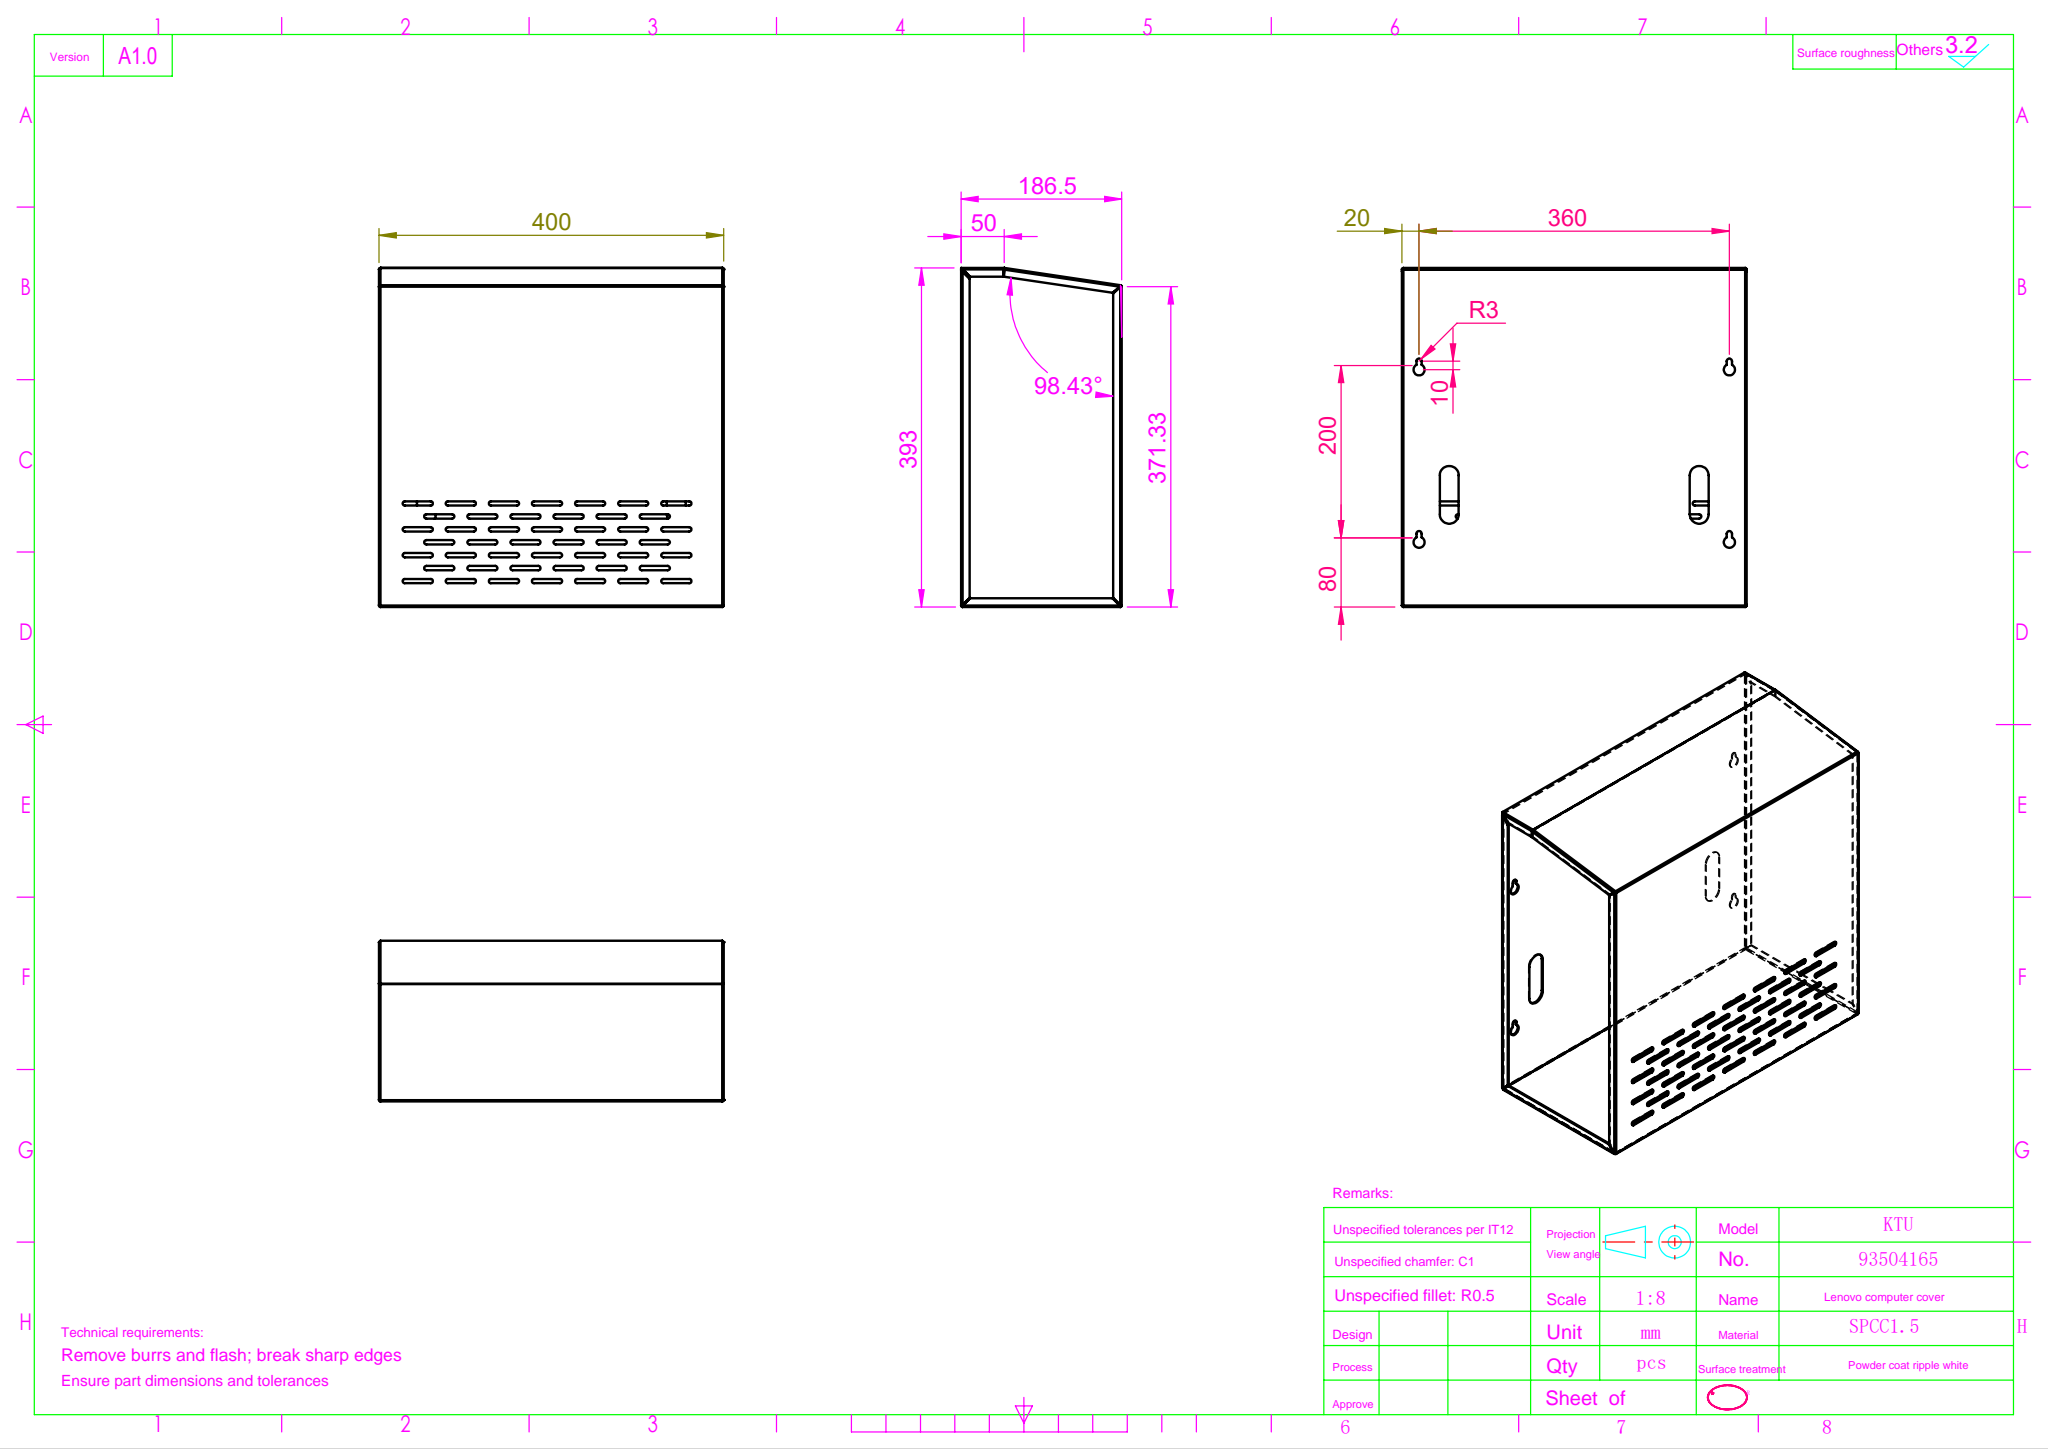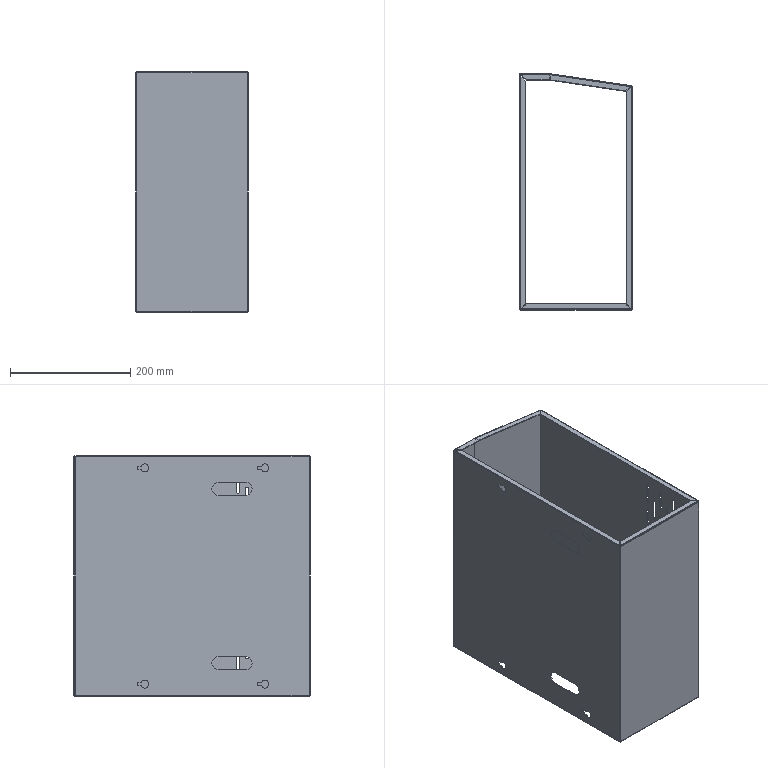Part | SolidWorks | features ICE 5, EdgeFlange 3, LPattern 2, FlatPattern 1, SMBaseFlange 1, SheetMetal 1 | 1 solid | 378 faces | box 186.5 x 393 x 400.001 mm | volume 689190 mm3 | cylinder 184 | plane 174 | spline 20 | commonest cylinder face diameters 5 x138 0.4 x14 3.4 x14 13 x8 22 x6 6 x4